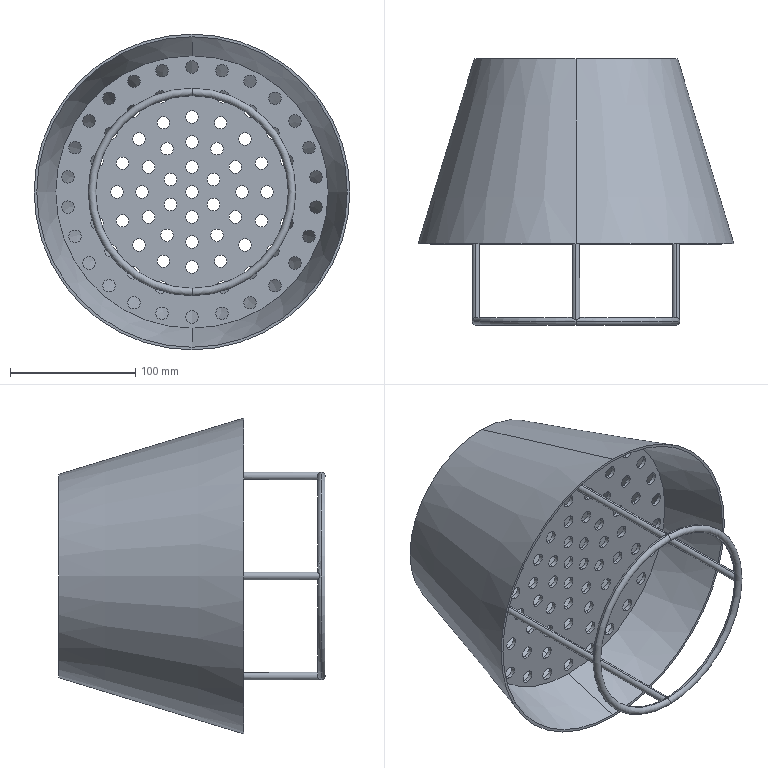Part | SolidWorks | features ICE 3, Revolution 2, Shell 1, Sweep 1 | 1 solid | 184 faces | box 252.5 x 213 x 252.5 mm | volume 319111 mm3 | cylinder 162 | plane 12 | cone 6 | torus 4 | commonest cylinder face diameters 10 x154 6 x8